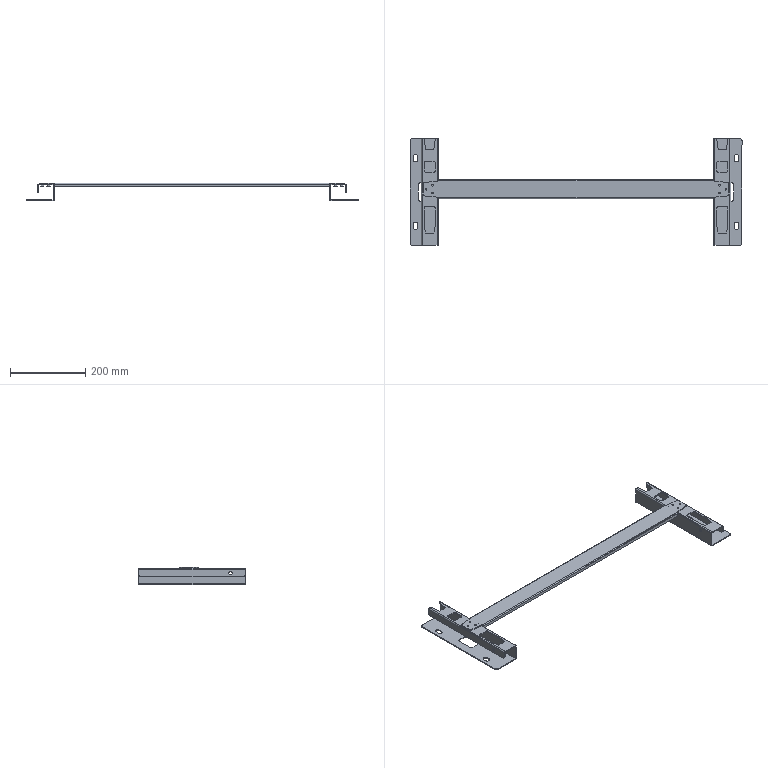Part | SolidWorks | 3 solids | 274 faces | box 885 x 285 x 47.5 mm | volume 349214 mm3 | plane 162 | cylinder 112 | commonest cylinder face diameters 12 x32 4.5 x24 6 x24 4 x12 1 x8 9 x8